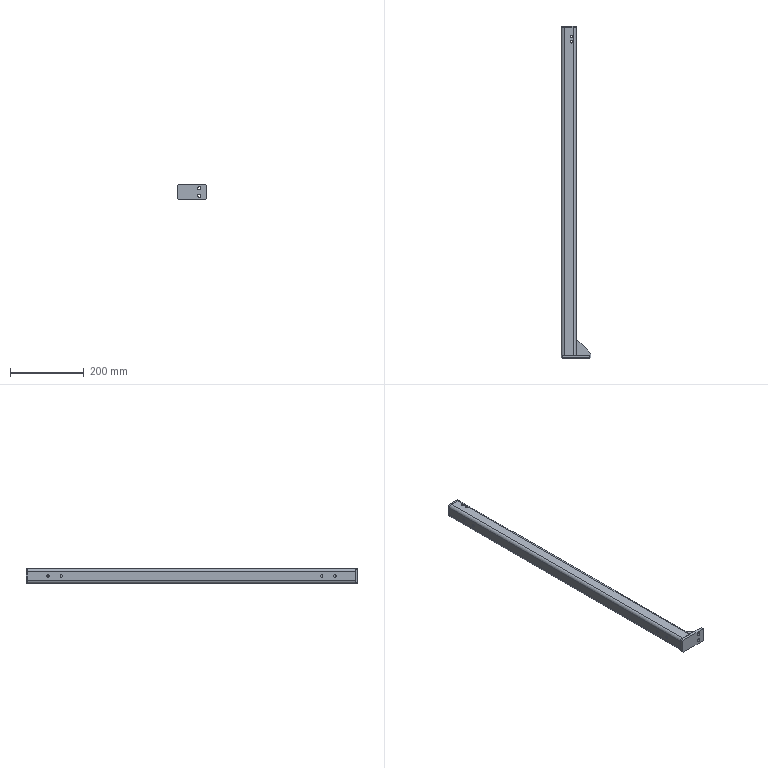Part | SolidWorks | features BaseBody 4 | 4 solids | 67 faces | box 80 x 903 x 40 mm | volume 514516 mm3 | cylinder 34 | plane 33 | commonest cylinder face diameters 6.8 x18 16 x8 8 x4 9 x4